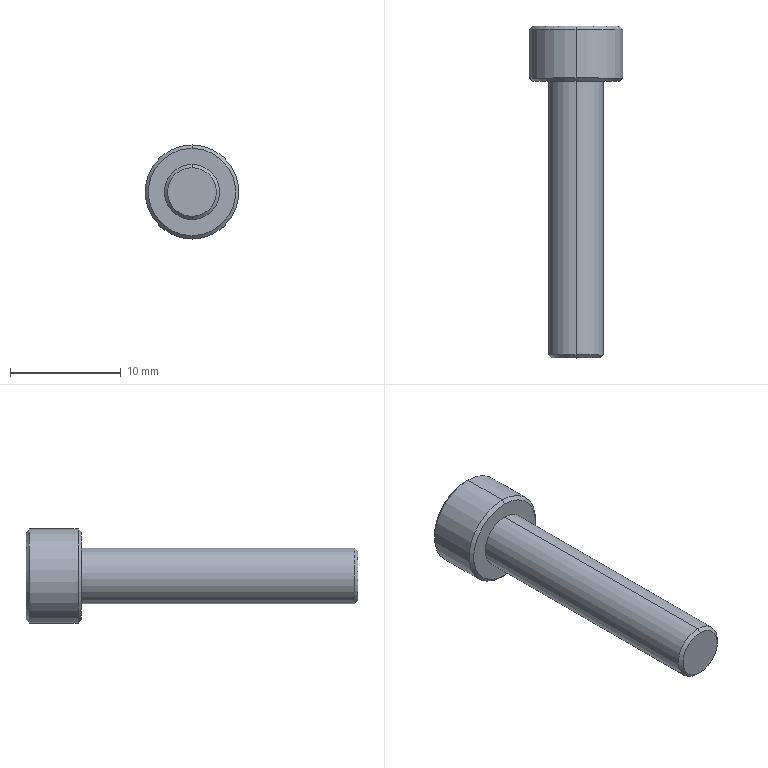Part | STEP file | Hex socket screw M5×25 | 1 solid | 28 faces | box 8.5 x 30 x 8.5 mm | volume 728.239 mm3 | plane 10 | cone 8 | spline 6 | cylinder 4 | commonest cylinder face diameters 5 x2 8.5 x2